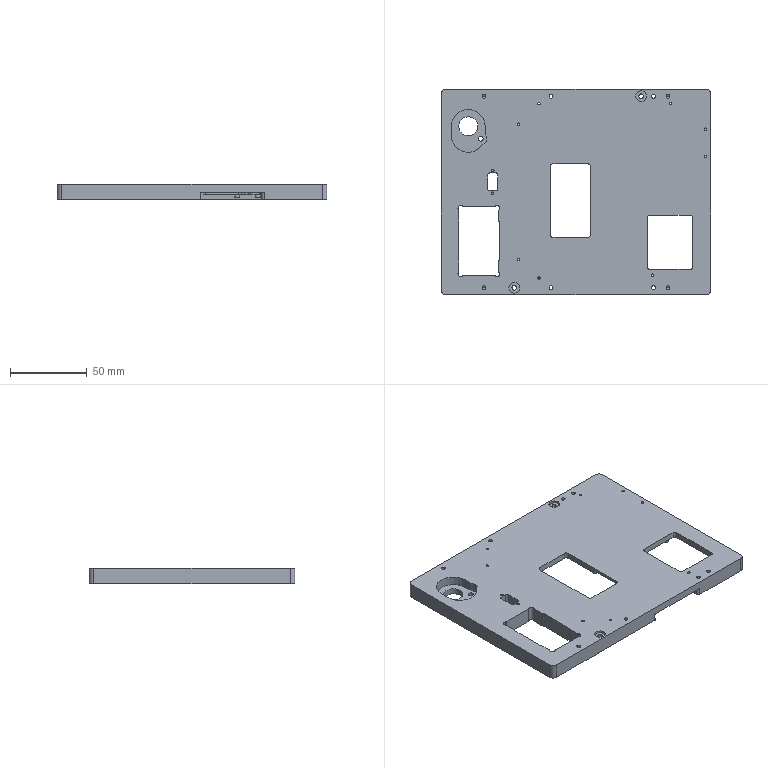NC program | NX | posted with a generic post | part box 176 x 134 x 10 mm
Lines 2899 to 3767 of 8914:
(ZLEVEL_PROFILE_COPY_COPY_COPY_1_COPY_COPY_1_COPY_COPY_COPY_1 , TOOL : D4)
N5748 T17 M6
N5750 G54
N5752 G17 G0 G90 X-55.013 Y2.813 S9500 M3
N5754 G43 Z30. H17
N5756 Z1.5
N5758 G94 G1 X-53.057 Y2.811 Z1.397 F1000.
N5760 X-53.058 Y2.859 Z1.395
N5762 X-53.05 Y10.431 Z0.998
N5764 X-55.55 Y10.434 Z0.867
N5766 X-55.59 Y10.436 Z0.865
N5768 X-55.598 Y2.85 Z0.467
N5770 X-55.601 Y2.814 Z0.466
N5772 X-53.057 Y2.811 Z0.332
N5774 X-53.058 Y2.859 Z0.33
N5776 X-53.05 Y10.431 Z-0.067
N5778 X-55.55 Y10.434 Z-0.198
N5780 X-55.59 Y10.436 Z-0.2
N5782 X-55.594 Y6.625 Z-0.4
N5784 X-55.598 Y2.85 F1500.
N5786 X-55.601 Y2.814
N5788 X-53.057 Y2.811
N5790 X-53.058 Y2.859
N5792 X-53.05 Y10.431
N5794 X-55.55 Y10.434
N5796 X-55.59 Y10.436
N5798 X-55.594 Y6.625
N5800 X-55.598 Y2.955 Z-0.496
N5802 Y2.814 Z-0.5
N5804 X-55.459 Z-0.504
N5806 X-53.201 Y2.811 Z-0.563
N5808 X-53.058 Z-0.567
N5810 Y2.949 Z-0.57
N5812 X-53.05 Y10.431 Z-0.767
N5814 X-54.32 Y10.433 Z-0.8
N5816 X-55.55 Y10.434
N5818 X-55.59 Y10.436
N5820 X-55.594 Y6.625
N5822 X-55.598 Y2.955 Z-0.896
N5824 Y2.814 Z-0.9
N5826 X-55.459 Z-0.904
N5828 X-53.201 Y2.811 Z-0.963
N5830 X-53.058 Z-0.967
N5832 Y2.949 Z-0.97
N5834 X-53.05 Y10.431 Z-1.167
N5836 X-54.32 Y10.433 Z-1.2
N5838 X-55.55 Y10.434
N5840 X-55.59 Y10.436
N5842 X-55.594 Y6.625
N5844 X-55.598 Y2.955 Z-1.296
N5846 Y2.814 Z-1.3
N5848 X-55.459 Z-1.304
N5850 X-53.201 Y2.811 Z-1.363
N5852 X-53.058 Z-1.367
N5854 Y2.949 Z-1.37
N5856 X-53.05 Y10.431 Z-1.567
N5858 X-54.32 Y10.433 Z-1.6
N5860 X-55.55 Y10.434
N5862 X-55.59 Y10.436
N5864 X-55.594 Y6.625
N5866 X-55.598 Y2.955 Z-1.696
N5868 Y2.814 Z-1.7
N5870 X-55.459 Z-1.704
N5872 X-53.201 Y2.811 Z-1.763
N5874 X-53.058 Z-1.767
N5876 Y2.949 Z-1.77
N5878 X-53.05 Y10.431 Z-1.967
N5880 X-54.32 Y10.433 Z-2.
N5882 X-55.55 Y10.434
N5884 X-55.59 Y10.436
N5886 X-55.594 Y6.625
N5888 X-55.598 Y2.955 Z-2.096
N5890 Y2.814 Z-2.1
N5892 X-55.459 Z-2.104
N5894 X-53.201 Y2.811 Z-2.163
N5896 X-53.058 Z-2.167
N5898 Y2.949 Z-2.17
N5900 X-53.05 Y10.431 Z-2.367
N5902 X-54.32 Y10.433 Z-2.4
N5904 X-55.55 Y10.434
N5906 X-55.59 Y10.436
N5908 X-55.594 Y6.625
N5910 X-55.598 Y2.955 Z-2.496
N5912 Y2.814 Z-2.5
N5914 X-55.459 Z-2.504
N5916 X-53.201 Y2.811 Z-2.563
N5918 X-53.058 Z-2.567
N5920 Y2.949 Z-2.57
N5922 X-53.05 Y10.431 Z-2.767
N5924 X-54.32 Y10.433 Z-2.8
N5926 X-55.55 Y10.434
N5928 X-55.59 Y10.436
N5930 X-55.594 Y6.625
N5932 X-55.598 Y2.955 Z-2.896
N5934 Y2.814 Z-2.9
N5936 X-55.459 Z-2.904
N5938 X-53.201 Y2.811 Z-2.963
N5940 X-53.058 Z-2.967
N5942 Y2.949 Z-2.97
N5944 X-53.05 Y10.431 Z-3.167
N5946 X-54.32 Y10.433 Z-3.2
N5948 X-55.55 Y10.434
N5950 X-55.59 Y10.436
N5952 X-55.594 Y6.625
N5954 X-55.598 Y2.955 Z-3.296
N5956 Y2.814 Z-3.3
N5958 X-55.459 Z-3.304
N5960 X-53.201 Y2.811 Z-3.363
N5962 X-53.058 Z-3.367
N5964 Y2.949 Z-3.37
N5966 X-53.05 Y10.431 Z-3.567
N5968 X-54.32 Y10.433 Z-3.6
N5970 X-55.55 Y10.434
N5972 X-55.59 Y10.436
N5974 X-55.594 Y6.625
N5976 X-55.598 Y2.955 Z-3.696
N5978 Y2.814 Z-3.7
N5980 X-55.459 Z-3.704
N5982 X-53.201 Y2.811 Z-3.763
N5984 X-53.058 Z-3.767
N5986 Y2.95 Z-3.77
N5988 X-53.05 Y10.431 Z-3.967
N5990 X-54.32 Y10.433 Z-4.
N5992 X-55.55 Y10.434
N5994 X-55.59 Y10.436
N5996 X-55.594 Y6.625
N5998 X-55.598 Y2.955 Z-4.096
N6000 Y2.814 Z-4.1
N6002 X-55.459 Z-4.104
N6004 X-53.201 Y2.811 Z-4.163
N6006 X-53.058 Z-4.167
N6008 Y2.95 Z-4.17
N6010 X-53.05 Y10.431 Z-4.367
N6012 X-54.32 Y10.433 Z-4.4
N6014 X-55.55 Y10.434
N6016 X-55.59 Y10.435
N6018 X-55.594 Y6.625
N6020 X-55.598 Y2.955 Z-4.496
N6022 Y2.814 Z-4.5
N6024 X-55.459 Z-4.504
N6026 X-53.201 Y2.811 Z-4.563
N6028 X-53.058 Z-4.567
N6030 Y2.95 Z-4.57
N6032 X-53.05 Y10.431 Z-4.767
N6034 X-54.32 Y10.433 Z-4.8
N6036 X-55.55 Y10.434
N6038 X-55.59 Y10.435
N6040 X-55.594 Y6.625
N6042 X-55.598 Y2.955 Z-4.896
N6044 Y2.814 Z-4.9
N6046 X-55.459 Z-4.904
N6048 X-53.201 Y2.811 Z-4.963
N6050 X-53.058 Z-4.967
N6052 Y2.95 Z-4.97
N6054 X-53.05 Y10.431 Z-5.167
N6056 X-54.32 Y10.433 Z-5.2
N6058 X-55.55 Y10.434
N6060 X-55.59 Y10.435
N6062 X-55.594 Y6.625
N6064 X-55.598 Y2.955 Z-5.296
N6066 Y2.814 Z-5.3
N6068 X-55.459 Z-5.304
N6070 X-53.2 Y2.811 Z-5.363
N6072 X-53.058 Z-5.367
N6074 Y2.95 Z-5.37
N6076 X-53.05 Y10.431 Z-5.567
N6078 X-54.32 Y10.433 Z-5.6
N6080 X-55.55 Y10.434
N6082 X-55.59 Y10.435
N6084 X-55.594 Y6.625
N6086 X-55.598 Y2.955 Z-5.696
N6088 Y2.814 Z-5.7
N6090 X-55.459 Z-5.704
N6092 X-53.2 Y2.811 Z-5.763
N6094 X-53.058 Z-5.767
N6096 Y2.95 Z-5.77
N6098 X-53.05 Y10.431 Z-5.967
N6100 X-54.32 Y10.433 Z-6.
N6102 X-55.55 Y10.434
N6104 X-55.59 Y10.435
N6106 X-55.594 Y6.625
N6108 X-55.598 Y2.955 Z-6.096
N6110 Y2.814 Z-6.1
N6112 X-55.459 Z-6.104
N6114 X-53.2 Y2.811 Z-6.163
N6116 X-53.058 Z-6.167
N6118 Y2.95 Z-6.17
N6120 X-53.05 Y10.431 Z-6.367
N6122 X-54.32 Y10.433 Z-6.4
N6124 X-55.55 Y10.434
N6126 X-55.59 Y10.435
N6128 X-55.594 Y6.625
N6130 X-55.598 Y2.955 Z-6.496
N6132 Y2.814 Z-6.5
N6134 X-55.459 Z-6.504
N6136 X-53.2 Y2.811 Z-6.563
N6138 X-53.058 Z-6.567
N6140 Y2.95 Z-6.57
N6142 X-53.05 Y10.431 Z-6.767
N6144 X-54.32 Y10.433 Z-6.8
N6146 X-55.55 Y10.434
N6148 X-55.59 Y10.435
N6150 X-55.594 Y6.625
N6152 X-55.598 Y2.955 Z-6.896
N6154 Y2.814 Z-6.9
N6156 X-55.459 Z-6.904
N6158 X-53.2 Y2.811 Z-6.963
N6160 X-53.058 Z-6.967
N6162 Y2.95 Z-6.97
N6164 X-53.05 Y10.431 Z-7.167
N6166 X-54.32 Y10.433 Z-7.2
N6168 X-55.55 Y10.434
N6170 X-55.59 Y10.435
N6172 X-55.594 Y6.625
N6174 X-55.598 Y2.955 Z-7.296
N6176 Y2.814 Z-7.3
N6178 X-55.459 Z-7.304
N6180 X-53.2 Y2.811 Z-7.363
N6182 X-53.058 Z-7.367
N6184 Y2.95 Z-7.37
N6186 X-53.05 Y10.431 Z-7.567
N6188 X-54.32 Y10.433 Z-7.6
N6190 X-55.55 Y10.434
N6192 X-55.59 Y10.435
N6194 X-55.594 Y6.625
N6196 X-55.598 Y2.955 Z-7.696
N6198 Y2.814 Z-7.7
N6200 X-55.458 Z-7.704
N6202 X-53.2 Y2.811 Z-7.763
N6204 X-53.058 Z-7.767
N6206 Y2.95 Z-7.77
N6208 X-53.05 Y10.431 Z-7.967
N6210 X-54.32 Y10.433 Z-8.
N6212 X-55.55 Y10.434
N6214 X-55.59 Y10.435
N6216 X-55.594 Y6.625
N6218 X-55.598 Y2.955 Z-8.096
N6220 Y2.814 Z-8.1
N6222 X-55.458 Z-8.104
N6224 X-53.2 Y2.811 Z-8.163
N6226 X-53.058 Z-8.167
N6228 Y2.95 Z-8.17
N6230 X-53.05 Y10.431 Z-8.367
N6232 X-54.32 Y10.433 Z-8.4
N6234 X-55.55 Y10.434
N6236 X-55.59 Y10.435
N6238 X-55.594 Y6.625
N6240 X-55.598 Y2.955 Z-8.496
N6242 Y2.814 Z-8.5
N6244 X-55.458 Z-8.504
N6246 X-53.2 Y2.811 Z-8.563
N6248 X-53.058 Z-8.567
N6250 Y2.95 Z-8.57
N6252 X-53.05 Y10.431 Z-8.767
N6254 X-54.32 Y10.433 Z-8.8
N6256 X-55.55 Y10.434
N6258 X-55.59 Y10.435
N6260 X-55.594 Y6.625
N6262 X-55.598 Y2.955 Z-8.896
N6264 Y2.814 Z-8.9
N6266 X-55.458 Z-8.904
N6268 X-53.2 Y2.811 Z-8.963
N6270 X-53.058 Z-8.967
N6272 Y2.95 Z-8.97
N6274 X-53.05 Y10.431 Z-9.167
N6276 X-54.32 Y10.433 Z-9.2
N6278 X-55.55 Y10.434
N6280 X-55.59 Y10.435
N6282 X-55.594 Y6.625
N6284 X-55.598 Y2.955 Z-9.296
N6286 Y2.814 Z-9.3
N6288 X-55.458 Z-9.304
N6290 X-53.2 Y2.811 Z-9.363
N6292 X-53.058 Z-9.367
N6294 Y2.95 Z-9.37
N6296 X-53.05 Y10.431 Z-9.567
N6298 X-54.32 Y10.433 Z-9.6
N6300 X-55.55 Y10.434
N6302 X-55.59 Y10.435
N6304 X-55.594 Y6.625
N6306 X-55.598 Y2.955 Z-9.696
N6308 Y2.814 Z-9.7
N6310 X-55.458 Z-9.704
N6312 X-53.2 Y2.811 Z-9.763
N6314 X-53.058 Z-9.767
N6316 Y2.95 Z-9.77
N6318 X-53.05 Y10.431 Z-9.967
N6320 X-54.32 Y10.433 Z-10.
N6322 X-55.55 Y10.434
N6324 X-55.59 Y10.435
N6326 X-55.598 Y2.85
N6328 X-55.599 Y2.814
N6330 X-53.057 Y2.811
N6332 X-53.058 Y2.859
N6334 X-53.05 Y10.431
N6336 X-54.32 Y10.433
N6338 Z-8.5
N6340 G0 Z30.
(ZLEVEL_PROFILE_COPY_COPY_COPY_1_COPY_COPY_1_COPY_COPY_COPY_1_COPY_COPY_COPY_1 )
N6342 X-62.776 Y32.833
N6344 Z-0.35
N6346 G1 X-62.157 Y32.572 F1000.
N6348 G3 X-61.76 Y32.622 R0.4
N6350 G2 X-61.068 Y33.109 R12. F1100.
N6352 G3 X-60.321 Y35.569 R2.
N6354 G2 X-60.625 Y36.358 R12.
N6356 G3 X-60.927 Y36.62 R0.4
N6358 G1 X-61.587 Y36.748
N6360 G0 X-62.776 Y32.833 Z-0.638
N6362 G1 X-62.157 Y32.572 F1000.
N6364 G3 X-61.76 Y32.622 R0.4
N6366 G2 X-61.068 Y33.109 R12. F1100.
N6368 G3 X-60.321 Y35.569 R2.
N6370 G2 X-60.625 Y36.358 R12.
N6372 G3 X-60.927 Y36.62 R0.4
N6374 G1 X-61.587 Y36.748
N6376 G0 X-62.776 Y32.833 Z-0.925
N6378 G1 X-62.157 Y32.572 F1000.
N6380 G3 X-61.76 Y32.622 R0.4
N6382 G2 X-61.068 Y33.109 R12. F1100.
N6384 G3 X-60.321 Y35.569 R2.
N6386 G2 X-60.625 Y36.358 R12.
N6388 G3 X-60.927 Y36.621 R0.4
N6390 G1 X-61.587 Y36.748
N6392 G0 X-62.776 Y32.833 Z-1.213
N6394 G1 X-62.157 Y32.572 F1000.
N6396 G3 X-61.76 Y32.621 R0.4
N6398 G2 X-61.068 Y33.109 R12. F1100.
N6400 G3 X-60.321 Y35.569 R2.
N6402 G2 X-60.625 Y36.359 R12.
N6404 G3 X-60.927 Y36.621 R0.4
N6406 G1 X-61.587 Y36.748
N6408 G0 X-62.776 Y32.832 Z-1.5
N6410 G1 X-62.157 Y32.572 F1000.
N6412 G3 X-61.76 Y32.621 R0.4
N6414 G2 X-61.068 Y33.109 R12. F1100.
N6416 G3 X-60.321 Y35.569 R2.
N6418 G2 X-60.625 Y36.359 R12.
N6420 G3 X-60.927 Y36.621 R0.4
N6422 G1 X-61.587 Y36.748
N6424 G0 X-62.776 Y32.832 Z-1.85
N6426 G1 X-62.157 Y32.572 F1000.
N6428 G3 X-61.76 Y32.621 R0.4
N6430 G2 X-61.068 Y33.109 R12. F1100.
N6432 G3 X-60.321 Y35.569 R2.
N6434 G2 X-60.625 Y36.359 R12.
N6436 G3 X-60.927 Y36.621 R0.4
N6438 G1 X-61.587 Y36.748
N6440 G0 X-62.776 Y32.832 Z-2.2
N6442 G1 X-62.157 Y32.571 F1000.
N6444 G3 X-61.76 Y32.621 R0.4
N6446 G2 X-61.068 Y33.109 R12. F1100.
N6448 G3 X-60.321 Y35.569 R2.
N6450 G2 X-60.625 Y36.359 R12.
N6452 G3 X-60.928 Y36.621 R0.4
N6454 G1 X-61.587 Y36.748
N6456 G0 X-62.776 Y32.832 Z-2.55
N6458 G1 X-62.157 Y32.571 F1000.
N6460 G3 X-61.76 Y32.621 R0.4
N6462 G2 X-61.068 Y33.109 R12. F1100.
N6464 G3 X-60.321 Y35.569 R2.
N6466 G2 X-60.625 Y36.359 R12.
N6468 G3 X-60.928 Y36.621 R0.4
N6470 G1 X-61.587 Y36.748
N6472 G0 X-62.776 Y32.832 Z-2.9
N6474 G1 X-62.157 Y32.571 F1000.
N6476 G3 X-61.76 Y32.621 R0.4
N6478 G2 X-61.068 Y33.109 R12. F1100.
N6480 G3 X-60.321 Y35.569 R2.
N6482 G2 X-60.625 Y36.359 R12.
N6484 G3 X-60.928 Y36.621 R0.4
N6486 G1 X-61.587 Y36.749
N6488 G0 X-62.777 Y32.832 Z-3.25
N6490 G1 X-62.157 Y32.571 F1000.
N6492 G3 X-61.761 Y32.621 R0.4
N6494 G2 X-61.068 Y33.109 R12. F1100.
N6496 G3 X-60.321 Y35.569 R2.
N6498 G2 X-60.625 Y36.359 R12.
N6500 G3 X-60.928 Y36.621 R0.4
N6502 G1 X-61.587 Y36.749
N6504 G0 X-62.777 Y32.832 Z-3.6
N6506 G1 X-62.158 Y32.571 F1000.
N6508 G3 X-61.761 Y32.621 R0.4
N6510 G2 X-61.068 Y33.109 R12. F1100.
N6512 G3 X-60.321 Y35.569 R2.
N6514 G2 X-60.625 Y36.359 R12.
N6516 G3 X-60.928 Y36.621 R0.4
N6518 G1 X-61.587 Y36.749
N6520 G0 X-62.777 Y32.832 Z-3.95
N6522 G1 X-62.158 Y32.571 F1000.
N6524 G3 X-61.761 Y32.621 R0.4
N6526 G2 X-61.068 Y33.109 R12. F1100.
N6528 G3 X-60.321 Y35.569 R2.
N6530 G2 X-60.626 Y36.359 R12.
N6532 G3 X-60.928 Y36.621 R0.4
N6534 G1 X-61.587 Y36.749
N6536 G0 X-62.777 Y32.832 Z-4.3
N6538 G1 X-62.158 Y32.571 F1000.
N6540 G3 X-61.761 Y32.621 R0.4
N6542 G2 X-61.068 Y33.109 R12. F1100.
N6544 G3 X-60.321 Y35.569 R2.
N6546 G2 X-60.626 Y36.359 R12.
N6548 G3 X-60.928 Y36.622 R0.4
N6550 G1 X-61.587 Y36.749
N6552 G0 X-62.777 Y32.832 Z-4.65
N6554 G1 X-62.158 Y32.571 F1000.
N6556 G3 X-61.761 Y32.621 R0.4
N6558 G2 X-61.068 Y33.109 R12. F1100.
N6560 G3 X-60.321 Y35.569 R2.
N6562 G2 X-60.626 Y36.36 R12.
N6564 G3 X-60.928 Y36.622 R0.4
N6566 G1 X-61.587 Y36.749
N6568 G0 X-62.777 Y32.832 Z-4.988
N6570 G1 X-62.158 Y32.571 F1000.
N6572 G3 X-61.761 Y32.621 R0.4
N6574 G2 X-61.068 Y33.109 R12. F1100.
N6576 G3 X-60.321 Y35.569 R2.
N6578 G2 X-60.626 Y36.36 R12.
N6580 G3 X-60.928 Y36.622 R0.4
N6582 G1 X-61.587 Y36.749
N6584 G0 X-62.777 Y32.832 Z-5.325
N6586 G1 X-62.158 Y32.571 F1000.
N6588 G3 X-61.761 Y32.621 R0.4
N6590 G2 X-61.068 Y33.109 R12. F1100.
N6592 G3 X-60.321 Y35.569 R2.
N6594 G2 X-60.626 Y36.36 R12.
N6596 G3 X-60.928 Y36.622 R0.4
N6598 G1 X-61.587 Y36.749
N6600 G0 X-62.777 Y32.832 Z-5.663
N6602 G1 X-62.158 Y32.571 F1000.
N6604 G3 X-61.761 Y32.621 R0.4
N6606 G2 X-61.068 Y33.109 R12. F1100.
N6608 G3 X-60.321 Y35.569 R2.
N6610 G2 X-60.626 Y36.36 R12.
N6612 G3 X-60.928 Y36.622 R0.4
N6614 G1 X-61.587 Y36.749
N6616 G0 X-62.777 Y32.832 Z-6.
N6618 G1 X-62.158 Y32.571 F1000.
N6620 G3 X-61.761 Y32.621 R0.4
N6622 G2 X-61.068 Y33.109 R12. F1100.
N6624 G3 X-60.321 Y35.569 R2.
N6626 G2 X-60.626 Y36.36 R12.
N6628 G3 X-60.928 Y36.622 R0.4
N6630 G1 X-61.587 Y36.75
N6632 G0 Z30.
N6634 X-73.702 Y-48.794
N6636 Z-0.35
N6638 G1 X-74.302 Y-49.14 F1000.
N6640 G3 X-74.502 Y-49.486 R0.4
N6642 G1 Y-51.789 F1100.
N6644 G2 X-74.686 Y-52.823 R3.
N6646 X-73.652 Y-52.639 R3.
N6648 G1 X-71.349
N6650 G3 X-71.003 Y-52.439 R0.4
N6652 G1 X-70.656 Y-51.839
N6654 G0 X-73.702 Y-48.794 Z-0.638
N6656 G1 X-74.302 Y-49.14 F1000.
N6658 G3 X-74.502 Y-49.486 R0.4
N6660 G1 Y-51.789 F1100.
N6662 G2 X-74.686 Y-52.823 R3.
N6664 X-73.652 Y-52.639 R3.
N6666 G1 X-71.349
N6668 G3 X-71.003 Y-52.439 R0.4
N6670 G1 X-70.656 Y-51.839
N6672 G0 X-73.702 Y-48.794 Z-0.925
N6674 G1 X-74.302 Y-49.14 F1000.
N6676 G3 X-74.502 Y-49.486 R0.4
N6678 G1 Y-51.789 F1100.
N6680 G2 X-74.686 Y-52.823 R3.
N6682 X-73.652 Y-52.639 R3.
N6684 G1 X-71.349
N6686 G3 X-71.003 Y-52.439 R0.4
N6688 G1 X-70.656 Y-51.839
N6690 G0 X-73.702 Y-48.794 Z-1.213
N6692 G1 X-74.302 Y-49.14 F1000.
N6694 G3 X-74.502 Y-49.486 R0.4
N6696 G1 Y-51.789 F1100.
N6698 G2 X-74.686 Y-52.823 R3.
N6700 X-73.652 Y-52.639 R3.
N6702 G1 X-71.349
N6704 G3 X-71.003 Y-52.439 R0.4
N6706 G1 X-70.656 Y-51.839
N6708 G0 X-73.702 Y-48.794 Z-1.5
N6710 G1 X-74.302 Y-49.14 F1000.
N6712 G3 X-74.502 Y-49.486 R0.4
N6714 G1 Y-51.789 F1100.
N6716 G2 X-74.686 Y-52.823 R3.
N6718 X-73.652 Y-52.639 R3.
N6720 G1 X-71.349
N6722 G3 X-71.003 Y-52.439 R0.4
N6724 G1 X-70.656 Y-51.839
N6726 G0 X-73.702 Y-48.794 Z-1.85
N6728 G1 X-74.302 Y-49.14 F1000.
N6730 G3 X-74.502 Y-49.486 R0.4
N6732 G1 Y-51.789 F1100.
N6734 G2 X-74.686 Y-52.823 R3.
N6736 X-73.652 Y-52.639 R3.
N6738 G1 X-71.349
N6740 G3 X-71.003 Y-52.439 R0.4
N6742 G1 X-70.656 Y-51.839
N6744 G0 X-73.702 Y-48.794 Z-2.2
N6746 G1 X-74.302 Y-49.14 F1000.
N6748 G3 X-74.502 Y-49.486 R0.4
N6750 G1 Y-51.789 F1100.
N6752 G2 X-74.686 Y-52.823 R3.
N6754 X-73.652 Y-52.639 R3.
N6756 G1 X-71.349
N6758 G3 X-71.003 Y-52.439 R0.4
N6760 G1 X-70.656 Y-51.839
N6762 G0 X-73.702 Y-48.794 Z-2.55
N6764 G1 X-74.302 Y-49.14 F1000.
N6766 G3 X-74.502 Y-49.486 R0.4
N6768 G1 Y-51.789 F1100.
N6770 G2 X-74.686 Y-52.823 R3.
N6772 X-73.652 Y-52.639 R3.
N6774 G1 X-71.349
N6776 G3 X-71.003 Y-52.439 R0.4
N6778 G1 X-70.656 Y-51.839
N6780 G0 X-73.702 Y-48.794 Z-2.9
N6782 G1 X-74.302 Y-49.14 F1000.
N6784 G3 X-74.502 Y-49.486 R0.4
N6786 G1 Y-51.789 F1100.
N6788 G2 X-74.686 Y-52.823 R3.
N6790 X-73.652 Y-52.639 R3.
N6792 G1 X-71.349
N6794 G3 X-71.003 Y-52.439 R0.4
N6796 G1 X-70.656 Y-51.839
N6798 G0 X-73.702 Y-48.794 Z-3.25
N6800 G1 X-74.302 Y-49.14 F1000.
N6802 G3 X-74.502 Y-49.486 R0.4
N6804 G1 Y-51.789 F1100.
N6806 G2 X-74.686 Y-52.823 R3.
N6808 X-73.652 Y-52.639 R3.
N6810 G1 X-71.349
N6812 G3 X-71.003 Y-52.439 R0.4
N6814 G1 X-70.656 Y-51.839
N6816 G0 X-73.702 Y-48.794 Z-3.6
N6818 G1 X-74.302 Y-49.14 F1000.
N6820 G3 X-74.502 Y-49.486 R0.4
N6822 G1 Y-51.789 F1100.
N6824 G2 X-74.686 Y-52.823 R3.
N6826 X-73.652 Y-52.639 R3.
N6828 G1 X-71.349
N6830 G3 X-71.003 Y-52.439 R0.4
N6832 G1 X-70.656 Y-51.839
N6834 G0 X-73.702 Y-48.794 Z-3.95
N6836 G1 X-74.302 Y-49.14 F1000.
N6838 G3 X-74.502 Y-49.486 R0.4
N6840 G1 Y-51.789 F1100.
N6842 G2 X-74.686 Y-52.823 R3.
N6844 X-73.652 Y-52.639 R3.
N6846 G1 X-71.349
N6848 G3 X-71.003 Y-52.439 R0.4
N6850 G1 X-70.656 Y-51.839
N6852 G0 X-73.702 Y-48.794 Z-4.3
N6854 G1 X-74.302 Y-49.14 F1000.
N6856 G3 X-74.502 Y-49.486 R0.4
N6858 G1 Y-51.789 F1100.
N6860 G2 X-74.686 Y-52.823 R3.
N6862 X-73.652 Y-52.639 R3.
N6864 G1 X-71.349
N6866 G3 X-71.003 Y-52.439 R0.4
N6868 G1 X-70.656 Y-51.839
N6870 G0 X-73.702 Y-48.794 Z-4.65
N6872 G1 X-74.302 Y-49.14 F1000.
N6874 G3 X-74.502 Y-49.486 R0.4
N6876 G1 Y-51.789 F1100.
N6878 G2 X-74.686 Y-52.823 R3.
N6880 X-73.652 Y-52.639 R3.
N6882 G1 X-71.349
N6884 G3 X-71.003 Y-52.439 R0.4
N6886 G1 X-70.656 Y-51.839
N6888 G0 X-73.702 Y-48.794 Z-4.988
N6890 G1 X-74.302 Y-49.14 F1000.
N6892 G3 X-74.502 Y-49.486 R0.4
N6894 G1 Y-51.789 F1100.
N6896 G2 X-74.686 Y-52.823 R3.
N6898 X-73.652 Y-52.639 R3.
N6900 G1 X-71.349
N6902 G3 X-71.003 Y-52.439 R0.4
N6904 G1 X-70.656 Y-51.839
N6906 G0 X-73.702 Y-48.794 Z-5.325
N6908 G1 X-74.302 Y-49.14 F1000.
N6910 G3 X-74.502 Y-49.486 R0.4
N6912 G1 Y-51.789 F1100.
N6914 G2 X-74.686 Y-52.823 R3.
N6916 X-73.652 Y-52.639 R3.
N6918 G1 X-71.349
N6920 G3 X-71.003 Y-52.439 R0.4
N6922 G1 X-70.656 Y-51.839
N6924 G0 X-73.702 Y-48.794 Z-5.663
N6926 G1 X-74.302 Y-49.14 F1000.
N6928 G3 X-74.502 Y-49.486 R0.4
N6930 G1 Y-51.789 F1100.
N6932 G2 X-74.686 Y-52.823 R3.
N6934 X-73.652 Y-52.639 R3.
N6936 G1 X-71.349
N6938 G3 X-71.003 Y-52.439 R0.4
N6940 G1 X-70.656 Y-51.839
N6942 G0 X-73.702 Y-48.794 Z-6.
N6944 G1 X-74.302 Y-49.14 F1000.
N6946 G3 X-74.502 Y-49.486 R0.4
N6948 G1 Y-51.789 F1100.
N6950 G2 X-74.686 Y-52.823 R3.
N6952 X-73.652 Y-52.639 R3.
N6954 G1 X-71.349
N6956 G3 X-71.003 Y-52.439 R0.4
N6958 G1 X-70.656 Y-51.839
N6960 G0 X-73.702 Y-48.794 Z-6.35
N6962 G1 X-74.302 Y-49.14 F1000.
N6964 G3 X-74.502 Y-49.486 R0.4
N6966 G1 Y-51.789 F1100.
N6968 G2 X-74.686 Y-52.823 R3.
N6970 X-73.652 Y-52.639 R3.
N6972 G1 X-71.349
N6974 G3 X-71.003 Y-52.439 R0.4
N6976 G1 X-70.656 Y-51.839
N6978 G0 X-73.702 Y-48.794 Z-6.7
N6980 G1 X-74.302 Y-49.14 F1000.
N6982 G3 X-74.502 Y-49.486 R0.4
N6984 G1 Y-51.789 F1100.
N6986 G2 X-74.686 Y-52.823 R3.
N6988 X-73.652 Y-52.639 R3.
N6990 G1 X-71.349
N6992 G3 X-71.003 Y-52.439 R0.4
N6994 G1 X-70.656 Y-51.839
N6996 G0 X-73.702 Y-48.794 Z-7.05
N6998 G1 X-74.302 Y-49.14 F1000.
N7000 G3 X-74.502 Y-49.486 R0.4
N7002 G1 Y-51.789 F1100.
N7004 G2 X-74.686 Y-52.823 R3.
N7006 X-73.652 Y-52.639 R3.
N7008 G1 X-71.349
N7010 G3 X-71.003 Y-52.439 R0.4
N7012 G1 X-70.656 Y-51.839
N7014 G0 X-73.702 Y-48.794 Z-7.4
N7016 G1 X-74.302 Y-49.14 F1000.
N7018 G3 X-74.502 Y-49.486 R0.4
N7020 G1 Y-51.789 F1100.
N7022 G2 X-74.686 Y-52.823 R3.
N7024 X-73.652 Y-52.639 R3.
N7026 G1 X-71.349
N7028 G3 X-71.003 Y-52.439 R0.4
N7030 G1 X-70.656 Y-51.839
N7032 G0 X-73.702 Y-48.794 Z-7.75
N7034 G1 X-74.302 Y-49.14 F1000.
N7036 G3 X-74.502 Y-49.486 R0.4
N7038 G1 Y-51.789 F1100.
N7040 G2 X-74.686 Y-52.823 R3.
N7042 X-73.652 Y-52.639 R3.
N7044 G1 X-71.349
N7046 G3 X-71.003 Y-52.439 R0.4
N7048 G1 X-70.656 Y-51.839
N7050 G0 X-73.702 Y-48.794 Z-8.1
N7052 G1 X-74.302 Y-49.14 F1000.
N7054 G3 X-74.502 Y-49.486 R0.4
N7056 G1 Y-51.789 F1100.
N7058 G2 X-74.686 Y-52.823 R3.
N7060 X-73.652 Y-52.639 R3.
N7062 G1 X-71.349
N7064 G3 X-71.003 Y-52.439 R0.4
N7066 G1 X-70.656 Y-51.839
N7068 G0 X-73.702 Y-48.794 Z-8.45
N7070 G1 X-74.302 Y-49.14 F1000.
N7072 G3 X-74.502 Y-49.486 R0.4
N7074 G1 Y-51.789 F1100.
N7076 G2 X-74.686 Y-52.823 R3.
N7078 X-73.652 Y-52.639 R3.
N7080 G1 X-71.349
N7082 G3 X-71.003 Y-52.439 R0.4
N7084 G1 X-70.656 Y-51.839
N7086 G0 X-73.702 Y-48.794 Z-8.8
N7088 G1 X-74.302 Y-49.14 F1000.
N7090 G3 X-74.502 Y-49.486 R0.4
N7092 G1 Y-51.789 F1100.
N7094 G2 X-74.686 Y-52.823 R3.
N7096 X-73.652 Y-52.639 R3.
N7098 G1 X-71.349
N7100 G3 X-71.003 Y-52.439 R0.4
N7102 G1 X-70.656 Y-51.839
N7104 G0 X-73.702 Y-48.794 Z-9.1
N7106 G1 X-74.302 Y-49.14 F1000.
N7108 G3 X-74.502 Y-49.486 R0.4
N7110 G1 Y-51.789 F1100.
N7112 G2 X-74.686 Y-52.823 R3.
N7114 X-73.652 Y-52.639 R3.
N7116 G1 X-71.349
N7118 G3 X-71.003 Y-52.439 R0.4
N7120 G1 X-70.656 Y-51.839
N7122 G0 X-73.702 Y-48.794 Z-9.4
N7124 G1 X-74.302 Y-49.14 F1000.
N7126 G3 X-74.502 Y-49.486 R0.4
N7128 G1 Y-51.789 F1100.
N7130 G2 X-74.686 Y-52.823 R3.
N7132 X-73.652 Y-52.639 R3.
N7134 G1 X-71.349
N7136 G3 X-71.003 Y-52.439 R0.4
N7138 G1 X-70.656 Y-51.839
N7140 G0 X-73.702 Y-48.794 Z-9.7
N7142 G1 X-74.302 Y-49.14 F1000.
N7144 G3 X-74.502 Y-49.486 R0.4
N7146 G1 Y-51.789 F1100.
N7148 G2 X-74.686 Y-52.823 R3.
N7150 X-73.652 Y-52.639 R3.
N7152 G1 X-71.349
N7154 G3 X-71.003 Y-52.439 R0.4
N7156 G1 X-70.656 Y-51.839
N7158 G0 X-73.702 Y-48.794 Z-10.
N7160 G1 X-74.302 Y-49.14 F1000.
N7162 G3 X-74.502 Y-49.486 R0.4
N7164 G1 Y-51.789 F1100.
N7166 G2 X-74.686 Y-52.823 R3.
N7168 X-73.652 Y-52.639 R3.
N7170 G1 X-71.349
N7172 G3 X-71.003 Y-52.439 R0.4
N7174 G1 X-70.656 Y-51.839
N7176 G0 Z30.
N7178 X-56.198
N7180 Z-0.35
N7182 G1 X-55.852 Y-52.439 F1000.
N7184 G3 X-55.505 Y-52.639 R0.4
N7186 G1 X-53.202 F1100.
N7188 G2 X-52.168 Y-52.823 R3.
N7190 X-52.352 Y-51.789 R3.
N7192 G1 Y-49.486
N7194 G3 X-52.552 Y-49.14 R0.4
N7196 G1 X-53.152 Y-48.794
N7198 G0 X-56.198 Y-51.839 Z-0.638
N7200 G1 X-55.852 Y-52.439 F1000.
N7202 G3 X-55.505 Y-52.639 R0.4
N7204 G1 X-53.202 F1100.
N7206 G2 X-52.168 Y-52.823 R3.
N7208 X-52.352 Y-51.789 R3.
N7210 G1 Y-49.486
N7212 G3 X-52.552 Y-49.14 R0.4
N7214 G1 X-53.152 Y-48.794
N7216 G0 X-56.198 Y-51.839 Z-0.925
N7218 G1 X-55.852 Y-52.439 F1000.
N7220 G3 X-55.505 Y-52.639 R0.4
N7222 G1 X-53.202 F1100.
N7224 G2 X-52.168 Y-52.823 R3.
N7226 X-52.352 Y-51.789 R3.
N7228 G1 Y-49.486
N7230 G3 X-52.552 Y-49.14 R0.4
N7232 G1 X-53.152 Y-48.794
N7234 G0 X-56.198 Y-51.839 Z-1.213
N7236 G1 X-55.852 Y-52.439 F1000.
N7238 G3 X-55.505 Y-52.639 R0.4
N7240 G1 X-53.202 F1100.
N7242 G2 X-52.168 Y-52.823 R3.
N7244 X-52.352 Y-51.789 R3.
N7246 G1 Y-49.486
N7248 G3 X-52.552 Y-49.14 R0.4
N7250 G1 X-53.152 Y-48.794
N7252 G0 X-56.198 Y-51.839 Z-1.5
N7254 G1 X-55.852 Y-52.439 F1000.
N7256 G3 X-55.505 Y-52.639 R0.4
N7258 G1 X-53.202 F1100.
N7260 G2 X-52.168 Y-52.823 R3.
N7262 X-52.352 Y-51.789 R3.
N7264 G1 Y-49.486
N7266 G3 X-52.552 Y-49.14 R0.4
N7268 G1 X-53.152 Y-48.794
N7270 G0 X-56.198 Y-51.839 Z-1.85
N7272 G1 X-55.852 Y-52.439 F1000.
N7274 G3 X-55.505 Y-52.639 R0.4
N7276 G1 X-53.202 F1100.
N7278 G2 X-52.168 Y-52.823 R3.
N7280 X-52.352 Y-51.789 R3.
N7282 G1 Y-49.486
N7284 G3 X-52.552 Y-49.14 R0.4
N7286 G1 X-53.152 Y-48.794
N7288 G0 X-56.198 Y-51.839 Z-2.2
N7290 G1 X-55.852 Y-52.439 F1000.
N7292 G3 X-55.505 Y-52.639 R0.4
N7294 G1 X-53.202 F1100.
N7296 G2 X-52.168 Y-52.823 R3.
N7298 X-52.352 Y-51.789 R3.
N7300 G1 Y-49.486
N7302 G3 X-52.552 Y-49.14 R0.4
N7304 G1 X-53.152 Y-48.794
N7306 G0 X-56.198 Y-51.839 Z-2.55
N7308 G1 X-55.852 Y-52.439 F1000.
N7310 G3 X-55.505 Y-52.639 R0.4
N7312 G1 X-53.202 F1100.
N7314 G2 X-52.168 Y-52.823 R3.
N7316 X-52.352 Y-51.789 R3.
N7318 G1 Y-49.486
N7320 G3 X-52.552 Y-49.14 R0.4
N7322 G1 X-53.152 Y-48.794
N7324 G0 X-56.198 Y-51.839 Z-2.9
N7326 G1 X-55.852 Y-52.439 F1000.
N7328 G3 X-55.505 Y-52.639 R0.4
N7330 G1 X-53.202 F1100.
N7332 G2 X-52.168 Y-52.823 R3.
N7334 X-52.352 Y-51.789 R3.
N7336 G1 Y-49.486
N7338 G3 X-52.552 Y-49.14 R0.4
N7340 G1 X-53.152 Y-48.794
N7342 G0 X-56.198 Y-51.839 Z-3.25
N7344 G1 X-55.852 Y-52.439 F1000.
N7346 G3 X-55.505 Y-52.639 R0.4
N7348 G1 X-53.202 F1100.
N7350 G2 X-52.168 Y-52.823 R3.
N7352 X-52.352 Y-51.789 R3.
N7354 G1 Y-49.486
N7356 G3 X-52.552 Y-49.14 R0.4
N7358 G1 X-53.152 Y-48.794
N7360 G0 X-56.198 Y-51.839 Z-3.6
N7362 G1 X-55.852 Y-52.439 F1000.
N7364 G3 X-55.505 Y-52.639 R0.4
N7366 G1 X-53.202 F1100.
N7368 G2 X-52.168 Y-52.823 R3.
N7370 X-52.352 Y-51.789 R3.
N7372 G1 Y-49.486
N7374 G3 X-52.552 Y-49.14 R0.4
N7376 G1 X-53.152 Y-48.794
N7378 G0 X-56.198 Y-51.839 Z-3.95
N7380 G1 X-55.852 Y-52.439 F1000.
N7382 G3 X-55.505 Y-52.639 R0.4
N7384 G1 X-53.202 F1100.
N7386 G2 X-52.168 Y-52.823 R3.
N7388 X-52.352 Y-51.789 R3.
N7390 G1 Y-49.486
N7392 G3 X-52.552 Y-49.14 R0.4
N7394 G1 X-53.152 Y-48.794
N7396 G0 X-56.198 Y-51.839 Z-4.3
N7398 G1 X-55.852 Y-52.439 F1000.
N7400 G3 X-55.505 Y-52.639 R0.4
N7402 G1 X-53.202 F1100.
N7404 G2 X-52.168 Y-52.823 R3.
N7406 X-52.352 Y-51.789 R3.
N7408 G1 Y-49.486
N7410 G3 X-52.552 Y-49.14 R0.4
N7412 G1 X-53.152 Y-48.794
N7414 G0 X-56.198 Y-51.839 Z-4.65
N7416 G1 X-55.852 Y-52.439 F1000.
N7418 G3 X-55.505 Y-52.639 R0.4
N7420 G1 X-53.202 F1100.
N7422 G2 X-52.168 Y-52.823 R3.
N7424 X-52.352 Y-51.789 R3.
N7426 G1 Y-49.486
N7428 G3 X-52.552 Y-49.14 R0.4
N7430 G1 X-53.152 Y-48.794
N7432 G0 X-56.198 Y-51.839 Z-4.988
N7434 G1 X-55.852 Y-52.439 F1000.
N7436 G3 X-55.505 Y-52.639 R0.4
N7438 G1 X-53.202 F1100.
N7440 G2 X-52.168 Y-52.823 R3.
N7442 X-52.352 Y-51.789 R3.
N7444 G1 Y-49.486
N7446 G3 X-52.552 Y-49.14 R0.4
N7448 G1 X-53.152 Y-48.794
N7450 G0 X-56.198 Y-51.839 Z-5.325
N7452 G1 X-55.852 Y-52.439 F1000.
N7454 G3 X-55.505 Y-52.639 R0.4
N7456 G1 X-53.202 F1100.
N7458 G2 X-52.168 Y-52.823 R3.
N7460 X-52.352 Y-51.789 R3.
N7462 G1 Y-49.486
N7464 G3 X-52.552 Y-49.14 R0.4
N7466 G1 X-53.152 Y-48.794
N7468 G0 X-56.198 Y-51.839 Z-5.663
N7470 G1 X-55.852 Y-52.439 F1000.
N7472 G3 X-55.505 Y-52.639 R0.4